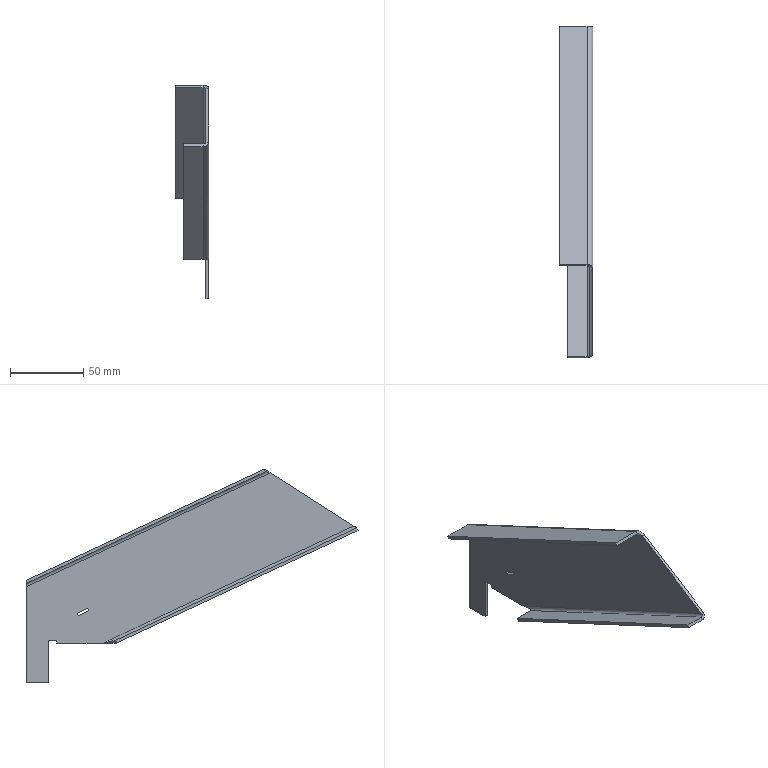Part | NX | features solid 2 | 1 solid | 31 faces | box 23 x 226.21 x 145.733 mm | volume 38939 mm3 | plane 23 | spline 4 | cylinder 4 | commonest cylinder face diameters 4 x2 8 x2
STEP:
#1=CARTESIAN_POINT('',(-258.,-1403.,125.937));
#2=VERTEX_POINT('',#1);
#3=CARTESIAN_POINT('',(-258.,-1388.,125.937));
#4=VERTEX_POINT('',#3);
#5=CARTESIAN_POINT('',(-258.,-1388.,125.937));
#6=DIRECTION('',(0.,1.,0.));
#7=VECTOR('',#6,1000.);
#8=LINE('',#5,#7);
#9=EDGE_CURVE('',#2,#4,#8,.T.);
#10=ORIENTED_EDGE('',*,*,#9,.F.);
#11=CARTESIAN_POINT('',(-260.,-1403.,125.937));
#12=VERTEX_POINT('',#11);
#13=CARTESIAN_POINT('',(-260.,-1403.,125.937));
#14=DIRECTION('',(1.,0.,0.));
#15=VECTOR('',#14,1000.);
#16=LINE('',#13,#15);
#17=EDGE_CURVE('',#12,#2,#16,.T.);
#18=ORIENTED_EDGE('',*,*,#17,.F.);
#19=CARTESIAN_POINT('',(-260.,-1388.,125.937));
#20=VERTEX_POINT('',#19);
#21=CARTESIAN_POINT('',(-260.,-1388.,125.937));
#22=DIRECTION('',(0.,1.,0.));
#23=VECTOR('',#22,1000.);
#24=LINE('',#21,#23);
#25=EDGE_CURVE('',#12,#20,#24,.T.);
#26=ORIENTED_EDGE('',*,*,#25,.T.);
#27=CARTESIAN_POINT('',(-260.,-1388.,125.937));
#28=DIRECTION('',(1.,0.,0.));
#29=VECTOR('',#28,1000.);
#30=LINE('',#27,#29);
#31=EDGE_CURVE('',#20,#4,#30,.T.);
#32=ORIENTED_EDGE('',*,*,#31,.T.);
#33=EDGE_LOOP('',(#10,#18,#26,#32));
#34=FACE_BOUND('',#33,.T.);
#35=CARTESIAN_POINT('',(-260.,-1388.,125.937));
#36=DIRECTION('',(0.,0.,-1.));
#37=DIRECTION('',(-1.,0.,0.));
#38=AXIS2_PLACEMENT_3D('',#35,#36,#37);
#39=PLANE('',#38);
#40=ADVANCED_FACE('',(#34),#39,.T.);
#41=CARTESIAN_POINT('',(-258.,-1403.,155.15));
#42=VERTEX_POINT('',#41);
#43=CARTESIAN_POINT('',(-258.,-1403.,155.15));
#44=DIRECTION('',(0.,0.,-1.));
#45=VECTOR('',#44,1000.);
#46=LINE('',#43,#45);
#47=EDGE_CURVE('',#42,#2,#46,.T.);
#48=ORIENTED_EDGE('',*,*,#47,.F.);
#49=CARTESIAN_POINT('',(-260.,-1403.,155.15));
#50=VERTEX_POINT('',#49);
#51=CARTESIAN_POINT('',(-260.,-1403.,155.15));
#52=DIRECTION('',(1.,0.,0.));
#53=VECTOR('',#52,1000.);
#54=LINE('',#51,#53);
#55=EDGE_CURVE('',#50,#42,#54,.T.);
#56=ORIENTED_EDGE('',*,*,#55,.F.);
#57=CARTESIAN_POINT('',(-260.,-1403.,155.15));
#58=DIRECTION('',(0.,0.,-1.));
#59=VECTOR('',#58,1000.);
#60=LINE('',#57,#59);
#61=EDGE_CURVE('',#50,#12,#60,.T.);
#62=ORIENTED_EDGE('',*,*,#61,.T.);
#63=ORIENTED_EDGE('',*,*,#17,.T.);
#64=EDGE_LOOP('',(#48,#56,#62,#63));
#65=FACE_BOUND('',#64,.T.);
#66=CARTESIAN_POINT('',(-260.,-1403.,155.15));
#67=DIRECTION('',(0.,-1.,0.));
#68=DIRECTION('',(0.,0.,-1.));
#69=AXIS2_PLACEMENT_3D('',#66,#67,#68);
#70=PLANE('',#69);
#71=ADVANCED_FACE('',(#65),#70,.T.);
#72=CARTESIAN_POINT('',(-260.,-1408.995,153.15));
#73=VERTEX_POINT('',#72);
#74=CARTESIAN_POINT('',(-260.,-1440.535,153.15));
#75=VERTEX_POINT('',#74);
#76=CARTESIAN_POINT('',(-260.,-1623.634,153.15));
#77=DIRECTION('',(0.,-1.,0.));
#78=VECTOR('',#77,1000.);
#79=LINE('',#76,#78);
#80=EDGE_CURVE('',#73,#75,#79,.T.);
#81=ORIENTED_EDGE('',*,*,#80,.F.);
#82=CARTESIAN_POINT('',(-258.,-1408.995,153.15));
#83=VERTEX_POINT('',#82);
#84=CARTESIAN_POINT('',(-258.,-1408.995,153.15));
#85=DIRECTION('',(1.,0.,0.));
#86=VECTOR('',#85,1000.);
#87=LINE('',#84,#86);
#88=EDGE_CURVE('',#73,#83,#87,.T.);
#89=ORIENTED_EDGE('',*,*,#88,.T.);
#90=CARTESIAN_POINT('',(-258.,-1440.535,153.15));
#91=VERTEX_POINT('',#90);
#92=CARTESIAN_POINT('',(-258.,-1623.634,153.15));
#93=DIRECTION('',(0.,-1.,0.));
#94=VECTOR('',#93,1000.);
#95=LINE('',#92,#94);
#96=EDGE_CURVE('',#83,#91,#95,.T.);
#97=ORIENTED_EDGE('',*,*,#96,.T.);
#98=CARTESIAN_POINT('',(-258.,-1440.535,153.15));
#99=DIRECTION('',(1.,0.,0.));
#100=VECTOR('',#99,1000.);
#101=LINE('',#98,#100);
#102=EDGE_CURVE('',#75,#91,#101,.T.);
#103=ORIENTED_EDGE('',*,*,#102,.F.);
#104=EDGE_LOOP('',(#81,#89,#97,#103));
#105=FACE_BOUND('',#104,.T.);
#106=CARTESIAN_POINT('',(-258.,-1623.634,153.15));
#107=DIRECTION('',(0.,0.,1.));
#108=DIRECTION('',(0.,-1.,0.));
#109=AXIS2_PLACEMENT_3D('',#106,#107,#108);
#110=PLANE('',#109);
#111=ADVANCED_FACE('',(#105),#110,.F.);
#112=CARTESIAN_POINT('',(-260.,-1408.995,155.15));
#113=VERTEX_POINT('',#112);
#114=CARTESIAN_POINT('',(-258.,-1408.995,155.15));
#115=VERTEX_POINT('',#114);
#116=CARTESIAN_POINT('',(-258.,-1408.995,155.15));
#117=DIRECTION('',(1.,0.,0.));
#118=VECTOR('',#117,1000.);
#119=LINE('',#116,#118);
#120=EDGE_CURVE('',#113,#115,#119,.T.);
#121=ORIENTED_EDGE('',*,*,#120,.T.);
#122=CARTESIAN_POINT('',(-258.,-1408.995,234.117));
#123=DIRECTION('',(0.,0.,-1.));
#124=VECTOR('',#123,1000.);
#125=LINE('',#122,#124);
#126=EDGE_CURVE('',#115,#83,#125,.T.);
#127=ORIENTED_EDGE('',*,*,#126,.T.);
#128=ORIENTED_EDGE('',*,*,#88,.F.);
#129=CARTESIAN_POINT('',(-260.,-1408.995,234.117));
#130=DIRECTION('',(0.,0.,-1.));
#131=VECTOR('',#130,1000.);
#132=LINE('',#129,#131);
#133=EDGE_CURVE('',#113,#73,#132,.T.);
#134=ORIENTED_EDGE('',*,*,#133,.F.);
#135=EDGE_LOOP('',(#121,#127,#128,#134));
#136=FACE_BOUND('',#135,.T.);
#137=CARTESIAN_POINT('',(-258.,-1408.995,234.117));
#138=DIRECTION('',(0.,-1.,0.));
#139=DIRECTION('',(-1.,0.,0.));
#140=AXIS2_PLACEMENT_3D('',#137,#138,#139);
#141=PLANE('',#140);
#142=ADVANCED_FACE('',(#136),#141,.F.);
#143=CARTESIAN_POINT('',(-260.,-1623.634,155.15));
#144=DIRECTION('',(0.,-1.,0.));
#145=VECTOR('',#144,1000.);
#146=LINE('',#143,#145);
#147=EDGE_CURVE('',#50,#113,#146,.T.);
#148=ORIENTED_EDGE('',*,*,#147,.F.);
#149=ORIENTED_EDGE('',*,*,#55,.T.);
#150=CARTESIAN_POINT('',(-258.,-1623.634,155.15));
#151=DIRECTION('',(0.,-1.,0.));
#152=VECTOR('',#151,1000.);
#153=LINE('',#150,#152);
#154=EDGE_CURVE('',#42,#115,#153,.T.);
#155=ORIENTED_EDGE('',*,*,#154,.T.);
#156=ORIENTED_EDGE('',*,*,#120,.F.);
#157=EDGE_LOOP('',(#148,#149,#155,#156));
#158=FACE_BOUND('',#157,.T.);
#159=CARTESIAN_POINT('',(-258.,-1623.634,155.15));
#160=DIRECTION('',(0.,0.,1.));
#161=DIRECTION('',(0.,-1.,0.));
#162=AXIS2_PLACEMENT_3D('',#159,#160,#161);
#163=PLANE('',#162);
#164=ADVANCED_FACE('',(#158),#163,.F.);
#165=CARTESIAN_POINT('',(-260.,-1388.,191.545));
#166=VERTEX_POINT('',#165);
#167=CARTESIAN_POINT('',(-258.,-1388.,191.545));
#168=VERTEX_POINT('',#167);
#169=CARTESIAN_POINT('',(-258.,-1388.,191.545));
#170=DIRECTION('',(1.,0.,0.));
#171=VECTOR('',#170,1000.);
#172=LINE('',#169,#171);
#173=EDGE_CURVE('',#166,#168,#172,.T.);
#174=ORIENTED_EDGE('',*,*,#173,.T.);
#175=CARTESIAN_POINT('',(-258.,-1388.,234.117));
#176=DIRECTION('',(0.,0.,-1.));
#177=VECTOR('',#176,1000.);
#178=LINE('',#175,#177);
#179=EDGE_CURVE('',#168,#4,#178,.T.);
#180=ORIENTED_EDGE('',*,*,#179,.T.);
#181=ORIENTED_EDGE('',*,*,#31,.F.);
#182=CARTESIAN_POINT('',(-260.,-1388.,234.117));
#183=DIRECTION('',(0.,0.,-1.));
#184=VECTOR('',#183,1000.);
#185=LINE('',#182,#184);
#186=EDGE_CURVE('',#166,#20,#185,.T.);
#187=ORIENTED_EDGE('',*,*,#186,.F.);
#188=EDGE_LOOP('',(#174,#180,#181,#187));
#189=FACE_BOUND('',#188,.T.);
#190=CARTESIAN_POINT('',(-258.,-1388.,234.117));
#191=DIRECTION('',(0.,-1.,0.));
#192=DIRECTION('',(-1.,0.,0.));
#193=AXIS2_PLACEMENT_3D('',#190,#191,#192);
#194=PLANE('',#193);
#195=ADVANCED_FACE('',(#189),#194,.F.);
#196=CARTESIAN_POINT('',(-262.,-1388.845,194.145));
#197=VERTEX_POINT('',#196);
#198=CARTESIAN_POINT('',(-262.,-1388.,195.958));
#199=VERTEX_POINT('',#198);
#200=CARTESIAN_POINT('',(-262.,-1388.,195.958));
#201=DIRECTION('',(0.,0.4226,0.9063));
#202=VECTOR('',#201,1000.);
#203=LINE('',#200,#202);
#204=EDGE_CURVE('',#197,#199,#203,.T.);
#205=ORIENTED_EDGE('',*,*,#204,.T.);
#206=CARTESIAN_POINT('',(-262.,-1388.,195.958));
#207=CARTESIAN_POINT('',(-259.657,-1388.,195.958));
#208=CARTESIAN_POINT('',(-258.,-1388.,194.13));
#209=CARTESIAN_POINT('',(-258.,-1388.,191.545));
#210=(BOUNDED_CURVE()B_SPLINE_CURVE(3,(#206,#207,#208,#209),.UNSPECIFIED.,.F.,.F.)B_SPLINE_CURVE_WITH_KNOTS((4,4),(3.142,4.712),.PIECEWISE_BEZIER_KNOTS.)CURVE()GEOMETRIC_REPRESENTATION_ITEM()RATIONAL_B_SPLINE_CURVE((1.,0.8047,0.8047,1.))REPRESENTATION_ITEM(''));
#211=EDGE_CURVE('',#199,#168,#210,.T.);
#212=ORIENTED_EDGE('',*,*,#211,.T.);
#213=ORIENTED_EDGE('',*,*,#173,.F.);
#214=CARTESIAN_POINT('',(-262.,-1388.845,194.145));
#215=CARTESIAN_POINT('',(-260.828,-1388.845,194.145));
#216=CARTESIAN_POINT('',(-260.,-1388.495,193.068));
#217=CARTESIAN_POINT('',(-260.,-1388.,191.545));
#218=(BOUNDED_CURVE()B_SPLINE_CURVE(3,(#214,#215,#216,#217),.UNSPECIFIED.,.F.,.F.)B_SPLINE_CURVE_WITH_KNOTS((4,4),(3.142,4.712),.PIECEWISE_BEZIER_KNOTS.)CURVE()GEOMETRIC_REPRESENTATION_ITEM()RATIONAL_B_SPLINE_CURVE((1.,0.8047,0.8047,1.))REPRESENTATION_ITEM(''));
#219=EDGE_CURVE('',#197,#166,#218,.T.);
#220=ORIENTED_EDGE('',*,*,#219,.F.);
#221=EDGE_LOOP('',(#205,#212,#213,#220));
#222=FACE_BOUND('',#221,.T.);
#223=CARTESIAN_POINT('',(-262.,-1388.,195.958));
#224=CARTESIAN_POINT('',(-262.,-1388.282,195.354));
#225=CARTESIAN_POINT('',(-262.,-1388.563,194.75));
#226=CARTESIAN_POINT('',(-262.,-1388.845,194.145));
#227=CARTESIAN_POINT('',(-260.,-1388.,195.958));
#228=CARTESIAN_POINT('',(-260.333,-1388.282,195.354));
#229=CARTESIAN_POINT('',(-260.667,-1388.563,194.75));
#230=CARTESIAN_POINT('',(-261.,-1388.845,194.145));
#231=CARTESIAN_POINT('',(-258.,-1388.,194.487));
#232=CARTESIAN_POINT('',(-258.667,-1388.188,194.084));
#233=CARTESIAN_POINT('',(-259.333,-1388.376,193.681));
#234=CARTESIAN_POINT('',(-260.,-1388.563,193.279));
#235=CARTESIAN_POINT('',(-258.,-1388.,191.545));
#236=CARTESIAN_POINT('',(-258.667,-1388.,191.545));
#237=CARTESIAN_POINT('',(-259.333,-1388.,191.545));
#238=CARTESIAN_POINT('',(-260.,-1388.,191.545));
#239=(BOUNDED_SURFACE()B_SPLINE_SURFACE(3,3,((#223,#224,#225,#226),(#227,#228,#229,#230),(#231,#232,#233,#234),(#235,#236,#237,#238)),.UNSPECIFIED.,.F.,.F.,.F.)B_SPLINE_SURFACE_WITH_KNOTS((4,4),(4,4),(0.5,0.75),(0.,1.),.PIECEWISE_BEZIER_KNOTS.)GEOMETRIC_REPRESENTATION_ITEM()RATIONAL_B_SPLINE_SURFACE(((1.,1.,1.,1.),(0.6667,0.6667,0.6667,0.6667),(0.5,0.5,0.5,0.5),(0.5,0.5,0.5,0.5)))REPRESENTATION_ITEM('')SURFACE());
#240=ADVANCED_FACE('',(#222),#239,.T.);
#241=CARTESIAN_POINT('',(-281.,-1388.845,194.145));
#242=VERTEX_POINT('',#241);
#243=CARTESIAN_POINT('',(-281.,-1388.,195.958));
#244=VERTEX_POINT('',#243);
#245=CARTESIAN_POINT('',(-281.,-1388.,195.958));
#246=DIRECTION('',(0.,0.4226,0.9063));
#247=VECTOR('',#246,1000.);
#248=LINE('',#245,#247);
#249=EDGE_CURVE('',#242,#244,#248,.T.);
#250=ORIENTED_EDGE('',*,*,#249,.T.);
#251=CARTESIAN_POINT('',(-258.,-1388.,195.958));
#252=DIRECTION('',(1.,0.,0.));
#253=VECTOR('',#252,1000.);
#254=LINE('',#251,#253);
#255=EDGE_CURVE('',#244,#199,#254,.T.);
#256=ORIENTED_EDGE('',*,*,#255,.T.);
#257=ORIENTED_EDGE('',*,*,#204,.F.);
#258=CARTESIAN_POINT('',(-258.,-1388.845,194.145));
#259=DIRECTION('',(1.,0.,0.));
#260=VECTOR('',#259,1000.);
#261=LINE('',#258,#260);
#262=EDGE_CURVE('',#242,#197,#261,.T.);
#263=ORIENTED_EDGE('',*,*,#262,.F.);
#264=EDGE_LOOP('',(#250,#256,#257,#263));
#265=FACE_BOUND('',#264,.T.);
#266=CARTESIAN_POINT('',(-258.,-1388.,195.958));
#267=DIRECTION('',(0.,-0.9063,0.4226));
#268=DIRECTION('',(-1.,0.,0.));
#269=AXIS2_PLACEMENT_3D('',#266,#267,#268);
#270=PLANE('',#269);
#271=ADVANCED_FACE('',(#265),#270,.F.);
#272=CARTESIAN_POINT('',(-262.,-1449.155,154.962));
#273=VERTEX_POINT('',#272);
#274=CARTESIAN_POINT('',(-262.,-1450.,153.15));
#275=VERTEX_POINT('',#274);
#276=CARTESIAN_POINT('',(-262.,-1450.,153.15));
#277=DIRECTION('',(0.,-0.4226,-0.9063));
#278=VECTOR('',#277,1000.);
#279=LINE('',#276,#278);
#280=EDGE_CURVE('',#273,#275,#279,.T.);
#281=ORIENTED_EDGE('',*,*,#280,.T.);
#282=CARTESIAN_POINT('',(-275.,-1450.,153.15));
#283=VERTEX_POINT('',#282);
#284=CARTESIAN_POINT('',(-275.,-1450.,153.15));
#285=DIRECTION('',(-1.,0.,0.));
#286=VECTOR('',#285,1000.);
#287=LINE('',#284,#286);
#288=EDGE_CURVE('',#275,#283,#287,.T.);
#289=ORIENTED_EDGE('',*,*,#288,.T.);
#290=CARTESIAN_POINT('',(-275.,-1449.155,154.962));
#291=VERTEX_POINT('',#290);
#292=CARTESIAN_POINT('',(-275.,-1450.,153.15));
#293=DIRECTION('',(0.,-0.4226,-0.9063));
#294=VECTOR('',#293,1000.);
#295=LINE('',#292,#294);
#296=EDGE_CURVE('',#291,#283,#295,.T.);
#297=ORIENTED_EDGE('',*,*,#296,.F.);
#298=CARTESIAN_POINT('',(-275.,-1449.155,154.962));
#299=DIRECTION('',(-1.,0.,0.));
#300=VECTOR('',#299,1000.);
#301=LINE('',#298,#300);
#302=EDGE_CURVE('',#273,#291,#301,.T.);
#303=ORIENTED_EDGE('',*,*,#302,.F.);
#304=EDGE_LOOP('',(#281,#289,#297,#303));
#305=FACE_BOUND('',#304,.T.);
#306=CARTESIAN_POINT('',(-275.,-1450.,153.15));
#307=DIRECTION('',(0.,-0.9063,0.4226));
#308=DIRECTION('',(-1.,0.,0.));
#309=AXIS2_PLACEMENT_3D('',#306,#307,#308);
#310=PLANE('',#309);
#311=ADVANCED_FACE('',(#305),#310,.F.);
#312=ORIENTED_EDGE('',*,*,#102,.T.);
#313=CARTESIAN_POINT('',(-258.,-1440.535,153.15));
#314=CARTESIAN_POINT('',(-258.,-1446.08,153.15));
#315=CARTESIAN_POINT('',(-259.657,-1450.,153.15));
#316=CARTESIAN_POINT('',(-262.,-1450.,153.15));
#317=(BOUNDED_CURVE()B_SPLINE_CURVE(3,(#313,#314,#315,#316),.UNSPECIFIED.,.F.,.F.)B_SPLINE_CURVE_WITH_KNOTS((4,4),(1.571,3.142),.PIECEWISE_BEZIER_KNOTS.)CURVE()GEOMETRIC_REPRESENTATION_ITEM()RATIONAL_B_SPLINE_CURVE((1.,0.8047,0.8047,1.))REPRESENTATION_ITEM(''));
#318=EDGE_CURVE('',#91,#275,#317,.T.);
#319=ORIENTED_EDGE('',*,*,#318,.T.);
#320=ORIENTED_EDGE('',*,*,#280,.F.);
#321=CARTESIAN_POINT('',(-260.,-1440.535,153.15));
#322=CARTESIAN_POINT('',(-260.,-1445.584,154.211));
#323=CARTESIAN_POINT('',(-260.828,-1449.155,154.962));
#324=CARTESIAN_POINT('',(-262.,-1449.155,154.962));
#325=(BOUNDED_CURVE()B_SPLINE_CURVE(3,(#321,#322,#323,#324),.UNSPECIFIED.,.F.,.F.)B_SPLINE_CURVE_WITH_KNOTS((4,4),(1.571,3.142),.PIECEWISE_BEZIER_KNOTS.)CURVE()GEOMETRIC_REPRESENTATION_ITEM()RATIONAL_B_SPLINE_CURVE((1.,0.8047,0.8047,1.))REPRESENTATION_ITEM(''));
#326=EDGE_CURVE('',#75,#273,#325,.T.);
#327=ORIENTED_EDGE('',*,*,#326,.F.);
#328=EDGE_LOOP('',(#312,#319,#320,#327));
#329=FACE_BOUND('',#328,.T.);
#330=CARTESIAN_POINT('',(-258.,-1440.535,153.15));
#331=CARTESIAN_POINT('',(-258.667,-1440.535,153.15));
#332=CARTESIAN_POINT('',(-259.333,-1440.535,153.15));
#333=CARTESIAN_POINT('',(-260.,-1440.535,153.15));
#334=CARTESIAN_POINT('',(-258.,-1446.845,153.15));
#335=CARTESIAN_POINT('',(-258.667,-1446.657,153.552));
#336=CARTESIAN_POINT('',(-259.333,-1446.469,153.955));
#337=CARTESIAN_POINT('',(-260.,-1446.282,154.358));
#338=CARTESIAN_POINT('',(-260.,-1450.,153.15));
#339=CARTESIAN_POINT('',(-260.333,-1449.718,153.754));
#340=CARTESIAN_POINT('',(-260.667,-1449.437,154.358));
#341=CARTESIAN_POINT('',(-261.,-1449.155,154.962));
#342=CARTESIAN_POINT('',(-262.,-1450.,153.15));
#343=CARTESIAN_POINT('',(-262.,-1449.718,153.754));
#344=CARTESIAN_POINT('',(-262.,-1449.437,154.358));
#345=CARTESIAN_POINT('',(-262.,-1449.155,154.962));
#346=(BOUNDED_SURFACE()B_SPLINE_SURFACE(3,3,((#330,#331,#332,#333),(#334,#335,#336,#337),(#338,#339,#340,#341),(#342,#343,#344,#345)),.UNSPECIFIED.,.F.,.F.,.F.)B_SPLINE_SURFACE_WITH_KNOTS((4,4),(4,4),(0.25,0.5),(0.,1.),.PIECEWISE_BEZIER_KNOTS.)GEOMETRIC_REPRESENTATION_ITEM()RATIONAL_B_SPLINE_SURFACE(((0.5,0.5,0.5,0.5),(0.5,0.5,0.5,0.5),(0.6667,0.6667,0.6667,0.6667),(1.,1.,1.,1.)))REPRESENTATION_ITEM('')SURFACE());
#347=ADVANCED_FACE('',(#329),#346,.T.);
#348=CARTESIAN_POINT('',(-262.,-1614.21,229.722));
#349=VERTEX_POINT('',#348);
#350=CARTESIAN_POINT('',(-258.,-1611.364,232.809));
#351=VERTEX_POINT('',#350);
#352=CARTESIAN_POINT('',(-262.,-1614.21,229.722));
#353=CARTESIAN_POINT('',(-259.657,-1614.21,229.722));
#354=CARTESIAN_POINT('',(-258.,-1613.031,231.));
#355=CARTESIAN_POINT('',(-258.,-1611.364,232.809));
#356=(BOUNDED_CURVE()B_SPLINE_CURVE(3,(#352,#353,#354,#355),.UNSPECIFIED.,.F.,.F.)B_SPLINE_CURVE_WITH_KNOTS((4,4),(3.142,4.712),.PIECEWISE_BEZIER_KNOTS.)CURVE()GEOMETRIC_REPRESENTATION_ITEM()RATIONAL_B_SPLINE_CURVE((1.,0.8047,0.8047,1.))REPRESENTATION_ITEM(''));
#357=EDGE_CURVE('',#349,#351,#356,.T.);
#358=ORIENTED_EDGE('',*,*,#357,.T.);
#359=CARTESIAN_POINT('',(-260.,-1611.364,232.809));
#360=VERTEX_POINT('',#359);
#361=CARTESIAN_POINT('',(-258.,-1611.364,232.809));
#362=DIRECTION('',(1.,0.,0.));
#363=VECTOR('',#362,1000.);
#364=LINE('',#361,#363);
#365=EDGE_CURVE('',#360,#351,#364,.T.);
#366=ORIENTED_EDGE('',*,*,#365,.F.);
#367=CARTESIAN_POINT('',(-262.,-1613.364,231.534));
#368=VERTEX_POINT('',#367);
#369=CARTESIAN_POINT('',(-262.,-1613.364,231.534));
#370=CARTESIAN_POINT('',(-260.828,-1613.364,231.534));
#371=CARTESIAN_POINT('',(-260.,-1612.536,232.062));
#372=CARTESIAN_POINT('',(-260.,-1611.364,232.809));
#373=(BOUNDED_CURVE()B_SPLINE_CURVE(3,(#369,#370,#371,#372),.UNSPECIFIED.,.F.,.F.)B_SPLINE_CURVE_WITH_KNOTS((4,4),(3.142,4.712),.PIECEWISE_BEZIER_KNOTS.)CURVE()GEOMETRIC_REPRESENTATION_ITEM()RATIONAL_B_SPLINE_CURVE((1.,0.8047,0.8047,1.))REPRESENTATION_ITEM(''));
#374=EDGE_CURVE('',#368,#360,#373,.T.);
#375=ORIENTED_EDGE('',*,*,#374,.F.);
#376=CARTESIAN_POINT('',(-262.,-1613.364,231.534));
#377=DIRECTION('',(0.,0.4226,0.9063));
#378=VECTOR('',#377,1000.);
#379=LINE('',#376,#378);
#380=EDGE_CURVE('',#349,#368,#379,.T.);
#381=ORIENTED_EDGE('',*,*,#380,.F.);
#382=EDGE_LOOP('',(#358,#366,#375,#381));
#383=FACE_BOUND('',#382,.T.);
#384=CARTESIAN_POINT('',(-262.,-1614.21,229.722));
#385=CARTESIAN_POINT('',(-262.,-1613.928,230.326));
#386=CARTESIAN_POINT('',(-262.,-1613.646,230.93));
#387=CARTESIAN_POINT('',(-262.,-1613.364,231.534));
#388=CARTESIAN_POINT('',(-260.,-1614.21,229.722));
#389=CARTESIAN_POINT('',(-260.333,-1613.928,230.326));
#390=CARTESIAN_POINT('',(-260.667,-1613.646,230.93));
#391=CARTESIAN_POINT('',(-261.,-1613.364,231.534));
#392=CARTESIAN_POINT('',(-258.,-1613.261,230.751));
#393=CARTESIAN_POINT('',(-258.667,-1613.073,231.153));
#394=CARTESIAN_POINT('',(-259.333,-1612.885,231.556));
#395=CARTESIAN_POINT('',(-260.,-1612.698,231.959));
#396=CARTESIAN_POINT('',(-258.,-1611.364,232.809));
#397=CARTESIAN_POINT('',(-258.667,-1611.364,232.809));
#398=CARTESIAN_POINT('',(-259.333,-1611.364,232.809));
#399=CARTESIAN_POINT('',(-260.,-1611.364,232.809));
#400=(BOUNDED_SURFACE()B_SPLINE_SURFACE(3,3,((#384,#385,#386,#387),(#388,#389,#390,#391),(#392,#393,#394,#395),(#396,#397,#398,#399)),.UNSPECIFIED.,.F.,.F.,.F.)B_SPLINE_SURFACE_WITH_KNOTS((4,4),(4,4),(0.5,0.75),(0.,1.),.PIECEWISE_BEZIER_KNOTS.)GEOMETRIC_REPRESENTATION_ITEM()RATIONAL_B_SPLINE_SURFACE(((1.,1.,1.,1.),(0.6667,0.6667,0.6667,0.6667),(0.5,0.5,0.5,0.5),(0.5,0.5,0.5,0.5)))REPRESENTATION_ITEM('')SURFACE());
#401=ADVANCED_FACE('',(#383),#400,.T.);
#402=ORIENTED_EDGE('',*,*,#380,.T.);
#403=CARTESIAN_POINT('',(-275.,-1613.364,231.534));
#404=VERTEX_POINT('',#403);
#405=CARTESIAN_POINT('',(-275.,-1613.364,231.534));
#406=DIRECTION('',(1.,0.,0.));
#407=VECTOR('',#406,1000.);
#408=LINE('',#405,#407);
#409=EDGE_CURVE('',#404,#368,#408,.T.);
#410=ORIENTED_EDGE('',*,*,#409,.F.);
#411=CARTESIAN_POINT('',(-275.,-1614.21,229.722));
#412=VERTEX_POINT('',#411);
#413=CARTESIAN_POINT('',(-275.,-1613.364,231.534));
#414=DIRECTION('',(0.,0.4226,0.9063));
#415=VECTOR('',#414,1000.);
#416=LINE('',#413,#415);
#417=EDGE_CURVE('',#412,#404,#416,.T.);
#418=ORIENTED_EDGE('',*,*,#417,.F.);
#419=CARTESIAN_POINT('',(-275.,-1614.21,229.722));
#420=DIRECTION('',(1.,0.,0.));
#421=VECTOR('',#420,1000.);
#422=LINE('',#419,#421);
#423=EDGE_CURVE('',#412,#349,#422,.T.);
#424=ORIENTED_EDGE('',*,*,#423,.T.);
#425=EDGE_LOOP('',(#402,#410,#418,#424));
#426=FACE_BOUND('',#425,.T.);
#427=CARTESIAN_POINT('',(-275.,-1613.364,231.534));
#428=DIRECTION('',(0.,0.9063,-0.4226));
#429=DIRECTION('',(-1.,0.,0.));
#430=AXIS2_PLACEMENT_3D('',#427,#428,#429);
#431=PLANE('',#430);
#432=ADVANCED_FACE('',(#426),#431,.F.);
#433=CARTESIAN_POINT('',(-260.,-1554.364,269.122));
#434=VERTEX_POINT('',#433);
#435=CARTESIAN_POINT('',(-262.,-1551.21,269.857));
#436=VERTEX_POINT('',#435);
#437=CARTESIAN_POINT('',(-260.,-1554.364,269.122));
#438=CARTESIAN_POINT('',(-260.,-1552.516,269.552));
#439=CARTESIAN_POINT('',(-260.828,-1551.21,269.857));
#440=CARTESIAN_POINT('',(-262.,-1551.21,269.857));
#441=(BOUNDED_CURVE()B_SPLINE_CURVE(3,(#437,#438,#439,#440),.UNSPECIFIED.,.F.,.F.)B_SPLINE_CURVE_WITH_KNOTS((4,4),(4.712,6.283),.PIECEWISE_BEZIER_KNOTS.)CURVE()GEOMETRIC_REPRESENTATION_ITEM()RATIONAL_B_SPLINE_CURVE((1.,0.8047,0.8047,1.))REPRESENTATION_ITEM(''));
#442=EDGE_CURVE('',#434,#436,#441,.T.);
#443=ORIENTED_EDGE('',*,*,#442,.F.);
#444=CARTESIAN_POINT('',(-258.,-1554.364,269.122));
#445=VERTEX_POINT('',#444);
#446=CARTESIAN_POINT('',(-258.,-1554.364,269.122));
#447=DIRECTION('',(1.,0.,0.));
#448=VECTOR('',#447,1000.);
#449=LINE('',#446,#448);
#450=EDGE_CURVE('',#434,#445,#449,.T.);
#451=ORIENTED_EDGE('',*,*,#450,.T.);
#452=CARTESIAN_POINT('',(-262.,-1550.364,271.67));
#453=VERTEX_POINT('',#452);
#454=CARTESIAN_POINT('',(-258.,-1554.364,269.122));
#455=CARTESIAN_POINT('',(-258.,-1552.021,270.614));
#456=CARTESIAN_POINT('',(-259.657,-1550.364,271.67));
#457=CARTESIAN_POINT('',(-262.,-1550.364,271.67));
#458=(BOUNDED_CURVE()B_SPLINE_CURVE(3,(#454,#455,#456,#457),.UNSPECIFIED.,.F.,.F.)B_SPLINE_CURVE_WITH_KNOTS((4,4),(4.712,6.283),.PIECEWISE_BEZIER_KNOTS.)CURVE()GEOMETRIC_REPRESENTATION_ITEM()RATIONAL_B_SPLINE_CURVE((1.,0.8047,0.8047,1.))REPRESENTATION_ITEM(''));
#459=EDGE_CURVE('',#445,#453,#458,.T.);
#460=ORIENTED_EDGE('',*,*,#459,.T.);
#461=CARTESIAN_POINT('',(-262.,-1550.364,271.67));
#462=DIRECTION('',(0.,0.4226,0.9063));
#463=VECTOR('',#462,1000.);
#464=LINE('',#461,#463);
#465=EDGE_CURVE('',#436,#453,#464,.T.);
#466=ORIENTED_EDGE('',*,*,#465,.F.);
#467=EDGE_LOOP('',(#443,#451,#460,#466));
#468=FACE_BOUND('',#467,.T.);
#469=CARTESIAN_POINT('',(-258.,-1554.364,269.122));
#470=CARTESIAN_POINT('',(-258.667,-1554.364,269.122));
#471=CARTESIAN_POINT('',(-259.333,-1554.364,269.122));
#472=CARTESIAN_POINT('',(-260.,-1554.364,269.122));
#473=CARTESIAN_POINT('',(-258.,-1551.698,270.82));
#474=CARTESIAN_POINT('',(-258.667,-1551.885,270.418));
#475=CARTESIAN_POINT('',(-259.333,-1552.073,270.015));
#476=CARTESIAN_POINT('',(-260.,-1552.261,269.612));
#477=CARTESIAN_POINT('',(-260.,-1550.364,271.67));
#478=CARTESIAN_POINT('',(-260.333,-1550.646,271.066));
#479=CARTESIAN_POINT('',(-260.667,-1550.928,270.461));
#480=CARTESIAN_POINT('',(-261.,-1551.21,269.857));
#481=CARTESIAN_POINT('',(-262.,-1550.364,271.67));
#482=CARTESIAN_POINT('',(-262.,-1550.646,271.066));
#483=CARTESIAN_POINT('',(-262.,-1550.928,270.461));
#484=CARTESIAN_POINT('',(-262.,-1551.21,269.857));
#485=(BOUNDED_SURFACE()B_SPLINE_SURFACE(3,3,((#469,#470,#471,#472),(#473,#474,#475,#476),(#477,#478,#479,#480),(#481,#482,#483,#484)),.UNSPECIFIED.,.F.,.F.,.F.)B_SPLINE_SURFACE_WITH_KNOTS((4,4),(4,4),(0.75,1.),(0.,1.),.PIECEWISE_BEZIER_KNOTS.)GEOMETRIC_REPRESENTATION_ITEM()RATIONAL_B_SPLINE_SURFACE(((0.5,0.5,0.5,0.5),(0.5,0.5,0.5,0.5),(0.6667,0.6667,0.6667,0.6667),(1.,1.,1.,1.)))REPRESENTATION_ITEM('')SURFACE());
#486=ADVANCED_FACE('',(#468),#485,.T.);
#487=ORIENTED_EDGE('',*,*,#365,.T.);
#488=CARTESIAN_POINT('',(-258.,-1619.499,227.626));
#489=DIRECTION('',(0.,0.8434,0.5373));
#490=VECTOR('',#489,1000.);
#491=LINE('',#488,#490);
#492=EDGE_CURVE('',#351,#445,#491,.T.);
#493=ORIENTED_EDGE('',*,*,#492,.T.);
#494=ORIENTED_EDGE('',*,*,#450,.F.);
#495=CARTESIAN_POINT('',(-260.,-1619.499,227.626));
#496=DIRECTION('',(0.,0.8434,0.5373));
#497=VECTOR('',#496,1000.);
#498=LINE('',#495,#497);
#499=EDGE_CURVE('',#360,#434,#498,.T.);
#500=ORIENTED_EDGE('',*,*,#499,.F.);
#501=EDGE_LOOP('',(#487,#493,#494,#500));
#502=FACE_BOUND('',#501,.T.);
#503=CARTESIAN_POINT('',(-258.,-1619.499,227.626));
#504=DIRECTION('',(0.,0.5373,-0.8434));
#505=DIRECTION('',(-1.,0.,0.));
#506=AXIS2_PLACEMENT_3D('',#503,#504,#505);
#507=PLANE('',#506);
#508=ADVANCED_FACE('',(#502),#507,.F.);
#509=ORIENTED_EDGE('',*,*,#465,.T.);
#510=CARTESIAN_POINT('',(-281.,-1550.364,271.67));
#511=VERTEX_POINT('',#510);
#512=CARTESIAN_POINT('',(-258.,-1550.364,271.67));
#513=DIRECTION('',(-1.,0.,0.));
#514=VECTOR('',#513,1000.);
#515=LINE('',#512,#514);
#516=EDGE_CURVE('',#453,#511,#515,.T.);
#517=ORIENTED_EDGE('',*,*,#516,.T.);
#518=CARTESIAN_POINT('',(-281.,-1551.21,269.857));
#519=VERTEX_POINT('',#518);
#520=CARTESIAN_POINT('',(-281.,-1550.364,271.67));
#521=DIRECTION('',(0.,0.4226,0.9063));
#522=VECTOR('',#521,1000.);
#523=LINE('',#520,#522);
#524=EDGE_CURVE('',#519,#511,#523,.T.);
#525=ORIENTED_EDGE('',*,*,#524,.F.);
#526=CARTESIAN_POINT('',(-258.,-1551.21,269.857));
#527=DIRECTION('',(-1.,0.,0.));
#528=VECTOR('',#527,1000.);
#529=LINE('',#526,#528);
#530=EDGE_CURVE('',#436,#519,#529,.T.);
#531=ORIENTED_EDGE('',*,*,#530,.F.);
#532=EDGE_LOOP('',(#509,#517,#525,#531));
#533=FACE_BOUND('',#532,.T.);
#534=CARTESIAN_POINT('',(-258.,-1550.364,271.67));
#535=DIRECTION('',(0.,0.9063,-0.4226));
#536=DIRECTION('',(-1.,0.,0.));
#537=AXIS2_PLACEMENT_3D('',#534,#535,#536);
#538=PLANE('',#537);
#539=ADVANCED_FACE('',(#533),#538,.F.);
#540=CARTESIAN_POINT('',(-258.,-1430.064,176.954));
#541=VERTEX_POINT('',#540);
#542=CARTESIAN_POINT('',(-258.,-1430.909,175.142));
#543=VERTEX_POINT('',#542);
#544=CARTESIAN_POINT('',(-258.,-1442.742,149.765));
#545=DIRECTION('',(0.,-0.4226,-0.9063));
#546=VECTOR('',#545,1000.);
#547=LINE('',#544,#546);
#548=EDGE_CURVE('',#541,#543,#547,.T.);
#549=ORIENTED_EDGE('',*,*,#548,.T.);
#550=CARTESIAN_POINT('',(-260.,-1430.909,175.142));
#551=VERTEX_POINT('',#550);
#552=CARTESIAN_POINT('',(47.821,-1430.909,175.142));
#553=DIRECTION('',(-1.,0.,0.));
#554=VECTOR('',#553,1000.);
#555=LINE('',#552,#554);
#556=EDGE_CURVE('',#543,#551,#555,.T.);
#557=ORIENTED_EDGE('',*,*,#556,.T.);
#558=CARTESIAN_POINT('',(-260.,-1430.064,176.954));
#559=VERTEX_POINT('',#558);
#560=CARTESIAN_POINT('',(-260.,-1430.064,176.954));
#561=DIRECTION('',(0.,0.4226,0.9063));
#562=VECTOR('',#561,1000.);
#563=LINE('',#560,#562);
#564=EDGE_CURVE('',#551,#559,#563,.T.);
#565=ORIENTED_EDGE('',*,*,#564,.T.);
#566=CARTESIAN_POINT('',(47.821,-1430.064,176.954));
#567=DIRECTION('',(-1.,0.,0.));
#568=VECTOR('',#567,1000.);
#569=LINE('',#566,#568);
#570=EDGE_CURVE('',#541,#559,#569,.T.);
#571=ORIENTED_EDGE('',*,*,#570,.F.);
#572=EDGE_LOOP('',(#549,#557,#565,#571));
#573=FACE_BOUND('',#572,.T.);
#574=CARTESIAN_POINT('',(47.821,-1430.064,176.954));
#575=DIRECTION('',(0.,-0.9063,0.4226));
#576=DIRECTION('',(-1.,0.,0.));
#577=AXIS2_PLACEMENT_3D('',#574,#575,#576);
#578=PLANE('',#577);
#579=ADVANCED_FACE('',(#573),#578,.F.);
#580=CARTESIAN_POINT('',(-258.,-1423.658,171.761));
#581=VERTEX_POINT('',#580);
#582=CARTESIAN_POINT('',(-258.,-1611.801,259.493));
#583=DIRECTION('',(0.,0.9063,-0.4226));
#584=VECTOR('',#583,1000.);
#585=LINE('',#582,#584);
#586=EDGE_CURVE('',#543,#581,#585,.T.);
#587=ORIENTED_EDGE('',*,*,#586,.T.);
#588=CARTESIAN_POINT('',(-260.,-1423.658,171.761));
#589=VERTEX_POINT('',#588);
#590=CARTESIAN_POINT('',(47.821,-1423.658,171.761));
#591=DIRECTION('',(-1.,0.,0.));
#592=VECTOR('',#591,1000.);
#593=LINE('',#590,#592);
#594=EDGE_CURVE('',#581,#589,#593,.T.);
#595=ORIENTED_EDGE('',*,*,#594,.T.);
#596=CARTESIAN_POINT('',(-260.,-1430.909,175.142));
#597=DIRECTION('',(0.,-0.9063,0.4226));
#598=VECTOR('',#597,1000.);
#599=LINE('',#596,#598);
#600=EDGE_CURVE('',#589,#551,#599,.T.);
#601=ORIENTED_EDGE('',*,*,#600,.T.);
#602=ORIENTED_EDGE('',*,*,#556,.F.);
#603=EDGE_LOOP('',(#587,#595,#601,#602));
#604=FACE_BOUND('',#603,.T.);
#605=CARTESIAN_POINT('',(47.821,-1430.909,175.142));
#606=DIRECTION('',(0.,-0.4226,-0.9063));
#607=DIRECTION('',(0.,-0.9063,0.4226));
#608=AXIS2_PLACEMENT_3D('',#605,#606,#607);
#609=PLANE('',#608);
#610=ADVANCED_FACE('',(#604),#609,.F.);
#611=CARTESIAN_POINT('',(-258.,-1422.813,173.574));
#612=VERTEX_POINT('',#611);
#613=CARTESIAN_POINT('',(-258.,-1435.492,146.384));
#614=DIRECTION('',(0.,0.4226,0.9063));
#615=VECTOR('',#614,1000.);
#616=LINE('',#613,#615);
#617=EDGE_CURVE('',#581,#612,#616,.T.);
#618=ORIENTED_EDGE('',*,*,#617,.T.);
#619=CARTESIAN_POINT('',(-260.,-1422.813,173.574));
#620=VERTEX_POINT('',#619);
#621=CARTESIAN_POINT('',(47.821,-1422.813,173.574));
#622=DIRECTION('',(-1.,0.,0.));
#623=VECTOR('',#622,1000.);
#624=LINE('',#621,#623);
#625=EDGE_CURVE('',#612,#620,#624,.T.);
#626=ORIENTED_EDGE('',*,*,#625,.T.);
#627=CARTESIAN_POINT('',(-260.,-1422.813,173.574));
#628=DIRECTION('',(0.,-0.4226,-0.9063));
#629=VECTOR('',#628,1000.);
#630=LINE('',#627,#629);
#631=EDGE_CURVE('',#620,#589,#630,.T.);
#632=ORIENTED_EDGE('',*,*,#631,.T.);
#633=ORIENTED_EDGE('',*,*,#594,.F.);
#634=EDGE_LOOP('',(#618,#626,#632,#633));
#635=FACE_BOUND('',#634,.T.);
#636=CARTESIAN_POINT('',(47.821,-1422.813,173.574));
#637=DIRECTION('',(0.,0.9063,-0.4226));
#638=DIRECTION('',(-1.,0.,0.));
#639=AXIS2_PLACEMENT_3D('',#636,#637,#638);
#640=PLANE('',#639);
#641=ADVANCED_FACE('',(#635),#640,.F.);
#642=CARTESIAN_POINT('',(-258.,-1610.956,261.306));
#643=DIRECTION('',(0.,-0.9063,0.4226));
#644=VECTOR('',#643,1000.);
#645=LINE('',#642,#644);
#646=EDGE_CURVE('',#612,#541,#645,.T.);
#647=ORIENTED_EDGE('',*,*,#646,.T.);
#648=ORIENTED_EDGE('',*,*,#570,.T.);
#649=CARTESIAN_POINT('',(-260.,-1430.064,176.954));
#650=DIRECTION('',(0.,0.9063,-0.4226));
#651=VECTOR('',#650,1000.);
#652=LINE('',#649,#651);
#653=EDGE_CURVE('',#559,#620,#652,.T.);
#654=ORIENTED_EDGE('',*,*,#653,.T.);
#655=ORIENTED_EDGE('',*,*,#625,.F.);
#656=EDGE_LOOP('',(#647,#648,#654,#655));
#657=FACE_BOUND('',#656,.T.);
#658=CARTESIAN_POINT('',(47.821,-1430.064,176.954));
#659=DIRECTION('',(0.,0.4226,0.9063));
#660=DIRECTION('',(1.,0.,0.));
#661=AXIS2_PLACEMENT_3D('',#658,#659,#660);
#662=PLANE('',#661);
#663=ADVANCED_FACE('',(#657),#662,.F.);
#664=CARTESIAN_POINT('',(-262.,-1622.789,235.929));
#665=DIRECTION('',(0.,0.9063,-0.4226));
#666=VECTOR('',#665,1000.);
#667=LINE('',#664,#666);
#668=EDGE_CURVE('',#368,#273,#667,.T.);
#669=ORIENTED_EDGE('',*,*,#668,.T.);
#670=ORIENTED_EDGE('',*,*,#302,.T.);
#671=CARTESIAN_POINT('',(-275.,-1622.789,235.929));
#672=DIRECTION('',(0.,0.9063,-0.4226));
#673=VECTOR('',#672,1000.);
#674=LINE('',#671,#673);
#675=EDGE_CURVE('',#404,#291,#674,.T.);
#676=ORIENTED_EDGE('',*,*,#675,.F.);
#677=ORIENTED_EDGE('',*,*,#409,.T.);
#678=EDGE_LOOP('',(#669,#670,#676,#677));
#679=FACE_BOUND('',#678,.T.);
#680=CARTESIAN_POINT('',(-275.,-1622.789,235.929));
#681=DIRECTION('',(0.,-0.4226,-0.9063));
#682=DIRECTION('',(0.,-0.9063,0.4226));
#683=AXIS2_PLACEMENT_3D('',#680,#681,#682);
#684=PLANE('',#683);
#685=ADVANCED_FACE('',(#679),#684,.F.);
#686=CARTESIAN_POINT('',(-260.,-1621.944,237.742));
#687=DIRECTION('',(0.,0.9063,-0.4226));
#688=VECTOR('',#687,1000.);
#689=LINE('',#686,#688);
#690=EDGE_CURVE('',#360,#75,#689,.T.);
#691=ORIENTED_EDGE('',*,*,#690,.T.);
#692=ORIENTED_EDGE('',*,*,#326,.T.);
#693=ORIENTED_EDGE('',*,*,#668,.F.);
#694=ORIENTED_EDGE('',*,*,#374,.T.);
#695=EDGE_LOOP('',(#691,#692,#693,#694));
#696=FACE_BOUND('',#695,.T.);
#697=CARTESIAN_POINT('',(-262.,-1621.944,237.742));
#698=DIRECTION('',(0.,0.9063,-0.4226));
#699=DIRECTION('',(1.,0.,0.));
#700=AXIS2_PLACEMENT_3D('',#697,#698,#699);
#701=CYLINDRICAL_SURFACE('',#700,2.);
#702=ADVANCED_FACE('',(#696),#701,.F.);
#703=CARTESIAN_POINT('',(-262.,-1597.009,291.214));
#704=DIRECTION('',(0.,0.9063,-0.4226));
#705=VECTOR('',#704,1000.);
#706=LINE('',#703,#705);
#707=EDGE_CURVE('',#436,#197,#706,.T.);
#708=ORIENTED_EDGE('',*,*,#707,.T.);
#709=ORIENTED_EDGE('',*,*,#219,.T.);
#710=CARTESIAN_POINT('',(-260.,-1597.854,289.401));
#711=DIRECTION('',(0.,0.9063,-0.4226));
#712=VECTOR('',#711,1000.);
#713=LINE('',#710,#712);
#714=EDGE_CURVE('',#434,#166,#713,.T.);
#715=ORIENTED_EDGE('',*,*,#714,.F.);
#716=ORIENTED_EDGE('',*,*,#442,.T.);
#717=EDGE_LOOP('',(#708,#709,#715,#716));
#718=FACE_BOUND('',#717,.T.);
#719=CARTESIAN_POINT('',(-262.,-1597.854,289.401));
#720=DIRECTION('',(0.,0.9063,-0.4226));
#721=DIRECTION('',(1.,0.,0.));
#722=AXIS2_PLACEMENT_3D('',#719,#720,#721);
#723=CYLINDRICAL_SURFACE('',#722,2.);
#724=ADVANCED_FACE('',(#718),#723,.F.);
#725=CARTESIAN_POINT('',(-281.,-1597.009,291.214));
#726=DIRECTION('',(0.,0.9063,-0.4226));
#727=VECTOR('',#726,1000.);
#728=LINE('',#725,#727);
#729=EDGE_CURVE('',#519,#242,#728,.T.);
#730=ORIENTED_EDGE('',*,*,#729,.T.);
#731=ORIENTED_EDGE('',*,*,#262,.T.);
#732=ORIENTED_EDGE('',*,*,#707,.F.);
#733=ORIENTED_EDGE('',*,*,#530,.T.);
#734=EDGE_LOOP('',(#730,#731,#732,#733));
#735=FACE_BOUND('',#734,.T.);
#736=CARTESIAN_POINT('',(-258.,-1597.009,291.214));
#737=DIRECTION('',(0.,0.4226,0.9063));
#738=DIRECTION('',(1.,0.,0.));
#739=AXIS2_PLACEMENT_3D('',#736,#737,#738);
#740=PLANE('',#739);
#741=ADVANCED_FACE('',(#735),#740,.F.);
#742=ORIENTED_EDGE('',*,*,#288,.F.);
#743=CARTESIAN_POINT('',(-262.,-1623.634,234.117));
#744=DIRECTION('',(0.,0.9063,-0.4226));
#745=VECTOR('',#744,1000.);
#746=LINE('',#743,#745);
#747=EDGE_CURVE('',#349,#275,#746,.T.);
#748=ORIENTED_EDGE('',*,*,#747,.F.);
#749=ORIENTED_EDGE('',*,*,#423,.F.);
#750=CARTESIAN_POINT('',(-275.,-1623.634,234.117));
#751=DIRECTION('',(0.,0.9063,-0.4226));
#752=VECTOR('',#751,1000.);
#753=LINE('',#750,#752);
#754=EDGE_CURVE('',#412,#283,#753,.T.);
#755=ORIENTED_EDGE('',*,*,#754,.T.);
#756=EDGE_LOOP('',(#742,#748,#749,#755));
#757=FACE_BOUND('',#756,.T.);
#758=CARTESIAN_POINT('',(-275.,-1623.634,234.117));
#759=DIRECTION('',(0.,-0.4226,-0.9063));
#760=DIRECTION('',(0.,-0.9063,0.4226));
#761=AXIS2_PLACEMENT_3D('',#758,#759,#760);
#762=PLANE('',#761);
#763=ADVANCED_FACE('',(#757),#762,.T.);
#764=ORIENTED_EDGE('',*,*,#318,.F.);
#765=CARTESIAN_POINT('',(-258.,-1621.944,237.742));
#766=DIRECTION('',(0.,0.9063,-0.4226));
#767=VECTOR('',#766,1000.);
#768=LINE('',#765,#767);
#769=EDGE_CURVE('',#351,#91,#768,.T.);
#770=ORIENTED_EDGE('',*,*,#769,.F.);
#771=ORIENTED_EDGE('',*,*,#357,.F.);
#772=ORIENTED_EDGE('',*,*,#747,.T.);
#773=EDGE_LOOP('',(#764,#770,#771,#772));
#774=FACE_BOUND('',#773,.T.);
#775=CARTESIAN_POINT('',(-262.,-1621.944,237.742));
#776=DIRECTION('',(0.,0.9063,-0.4226));
#777=DIRECTION('',(1.,0.,0.));
#778=AXIS2_PLACEMENT_3D('',#775,#776,#777);
#779=CYLINDRICAL_SURFACE('',#778,4.);
#780=ADVANCED_FACE('',(#774),#779,.T.);
#781=ORIENTED_EDGE('',*,*,#211,.F.);
#782=CARTESIAN_POINT('',(-262.,-1596.164,293.027));
#783=DIRECTION('',(0.,0.9063,-0.4226));
#784=VECTOR('',#783,1000.);
#785=LINE('',#782,#784);
#786=EDGE_CURVE('',#453,#199,#785,.T.);
#787=ORIENTED_EDGE('',*,*,#786,.F.);
#788=ORIENTED_EDGE('',*,*,#459,.F.);
#789=CARTESIAN_POINT('',(-258.,-1597.854,289.401));
#790=DIRECTION('',(0.,0.9063,-0.4226));
#791=VECTOR('',#790,1000.);
#792=LINE('',#789,#791);
#793=EDGE_CURVE('',#445,#168,#792,.T.);
#794=ORIENTED_EDGE('',*,*,#793,.T.);
#795=EDGE_LOOP('',(#781,#787,#788,#794));
#796=FACE_BOUND('',#795,.T.);
#797=CARTESIAN_POINT('',(-262.,-1597.854,289.401));
#798=DIRECTION('',(0.,0.9063,-0.4226));
#799=DIRECTION('',(1.,0.,0.));
#800=AXIS2_PLACEMENT_3D('',#797,#798,#799);
#801=CYLINDRICAL_SURFACE('',#800,4.);
#802=ADVANCED_FACE('',(#796),#801,.T.);
#803=ORIENTED_EDGE('',*,*,#255,.F.);
#804=CARTESIAN_POINT('',(-281.,-1596.164,293.027));
#805=DIRECTION('',(0.,0.9063,-0.4226));
#806=VECTOR('',#805,1000.);
#807=LINE('',#804,#806);
#808=EDGE_CURVE('',#511,#244,#807,.T.);
#809=ORIENTED_EDGE('',*,*,#808,.F.);
#810=ORIENTED_EDGE('',*,*,#516,.F.);
#811=ORIENTED_EDGE('',*,*,#786,.T.);
#812=EDGE_LOOP('',(#803,#809,#810,#811));
#813=FACE_BOUND('',#812,.T.);
#814=CARTESIAN_POINT('',(-258.,-1596.164,293.027));
#815=DIRECTION('',(0.,0.4226,0.9063));
#816=DIRECTION('',(1.,0.,0.));
#817=AXIS2_PLACEMENT_3D('',#814,#815,#816);
#818=PLANE('',#817);
#819=ADVANCED_FACE('',(#813),#818,.T.);
#820=ORIENTED_EDGE('',*,*,#249,.F.);
#821=ORIENTED_EDGE('',*,*,#729,.F.);
#822=ORIENTED_EDGE('',*,*,#524,.T.);
#823=ORIENTED_EDGE('',*,*,#808,.T.);
#824=EDGE_LOOP('',(#820,#821,#822,#823));
#825=FACE_BOUND('',#824,.T.);
#826=CARTESIAN_POINT('',(-281.,-1596.164,293.027));
#827=DIRECTION('',(1.,0.,0.));
#828=DIRECTION('',(0.,0.,-1.));
#829=AXIS2_PLACEMENT_3D('',#826,#827,#828);
#830=PLANE('',#829);
#831=ADVANCED_FACE('',(#825),#830,.F.);
#832=ORIENTED_EDGE('',*,*,#296,.T.);
#833=ORIENTED_EDGE('',*,*,#754,.F.);
#834=ORIENTED_EDGE('',*,*,#417,.T.);
#835=ORIENTED_EDGE('',*,*,#675,.T.);
#836=EDGE_LOOP('',(#832,#833,#834,#835));
#837=FACE_BOUND('',#836,.T.);
#838=CARTESIAN_POINT('',(-275.,-1623.634,234.117));
#839=DIRECTION('',(-1.,0.,0.));
#840=DIRECTION('',(0.,1.,0.));
#841=AXIS2_PLACEMENT_3D('',#838,#839,#840);
#842=PLANE('',#841);
#843=ADVANCED_FACE('',(#837),#842,.T.);
#844=ORIENTED_EDGE('',*,*,#631,.F.);
#845=ORIENTED_EDGE('',*,*,#653,.F.);
#846=ORIENTED_EDGE('',*,*,#564,.F.);
#847=ORIENTED_EDGE('',*,*,#600,.F.);
#848=EDGE_LOOP('',(#844,#845,#846,#847));
#849=FACE_BOUND('',#848,.T.);
#850=ORIENTED_EDGE('',*,*,#714,.T.);
#851=ORIENTED_EDGE('',*,*,#186,.T.);
#852=ORIENTED_EDGE('',*,*,#25,.F.);
#853=ORIENTED_EDGE('',*,*,#61,.F.);
#854=ORIENTED_EDGE('',*,*,#147,.T.);
#855=ORIENTED_EDGE('',*,*,#133,.T.);
#856=ORIENTED_EDGE('',*,*,#80,.T.);
#857=ORIENTED_EDGE('',*,*,#690,.F.);
#858=ORIENTED_EDGE('',*,*,#499,.T.);
#859=EDGE_LOOP('',(#850,#851,#852,#853,#854,#855,#856,#857,#858));
#860=FACE_BOUND('',#859,.T.);
#861=CARTESIAN_POINT('',(-260.,-1623.634,234.117));
#862=DIRECTION('',(1.,0.,0.));
#863=DIRECTION('',(0.,0.,-1.));
#864=AXIS2_PLACEMENT_3D('',#861,#862,#863);
#865=PLANE('',#864);
#866=ADVANCED_FACE('',(#849,#860),#865,.F.);
#867=ORIENTED_EDGE('',*,*,#646,.F.);
#868=ORIENTED_EDGE('',*,*,#617,.F.);
#869=ORIENTED_EDGE('',*,*,#586,.F.);
#870=ORIENTED_EDGE('',*,*,#548,.F.);
#871=EDGE_LOOP('',(#867,#868,#869,#870));
#872=FACE_BOUND('',#871,.T.);
#873=ORIENTED_EDGE('',*,*,#179,.F.);
#874=ORIENTED_EDGE('',*,*,#793,.F.);
#875=ORIENTED_EDGE('',*,*,#492,.F.);
#876=ORIENTED_EDGE('',*,*,#769,.T.);
#877=ORIENTED_EDGE('',*,*,#96,.F.);
#878=ORIENTED_EDGE('',*,*,#126,.F.);
#879=ORIENTED_EDGE('',*,*,#154,.F.);
#880=ORIENTED_EDGE('',*,*,#47,.T.);
#881=ORIENTED_EDGE('',*,*,#9,.T.);
#882=EDGE_LOOP('',(#873,#874,#875,#876,#877,#878,#879,#880,#881));
#883=FACE_BOUND('',#882,.T.);
#884=CARTESIAN_POINT('',(-258.,-1623.634,234.117));
#885=DIRECTION('',(1.,0.,0.));
#886=DIRECTION('',(0.,0.,-1.));
#887=AXIS2_PLACEMENT_3D('',#884,#885,#886);
#888=PLANE('',#887);
#889=ADVANCED_FACE('',(#872,#883),#888,.T.);
#890=CLOSED_SHELL('',(#40,#71,#111,#142,#164,#195,#240,#271,#311,#347,#401,#432,#486,#508,#539,#579,#610,#641,#663,#685,#702,#724,#741,#763,#780,#802,#819,#831,#843,#866,#889));
#891=MANIFOLD_SOLID_BREP('',#890);
#892=(LENGTH_UNIT()NAMED_UNIT(*)SI_UNIT(.MILLI.,.METRE.));
#893=UNCERTAINTY_MEASURE_WITH_UNIT(LENGTH_MEASURE(0.00001),#892,'','');
#894=(NAMED_UNIT(*)PLANE_ANGLE_UNIT()SI_UNIT($,.RADIAN.));
#895=(NAMED_UNIT(*)SI_UNIT($,.STERADIAN.)SOLID_ANGLE_UNIT());
#896=(GEOMETRIC_REPRESENTATION_CONTEXT(3)GLOBAL_UNCERTAINTY_ASSIGNED_CONTEXT((#893))GLOBAL_UNIT_ASSIGNED_CONTEXT((#892,#894,#895))REPRESENTATION_CONTEXT('',''));
#897=ADVANCED_BREP_SHAPE_REPRESENTATION('',(#891),#896);